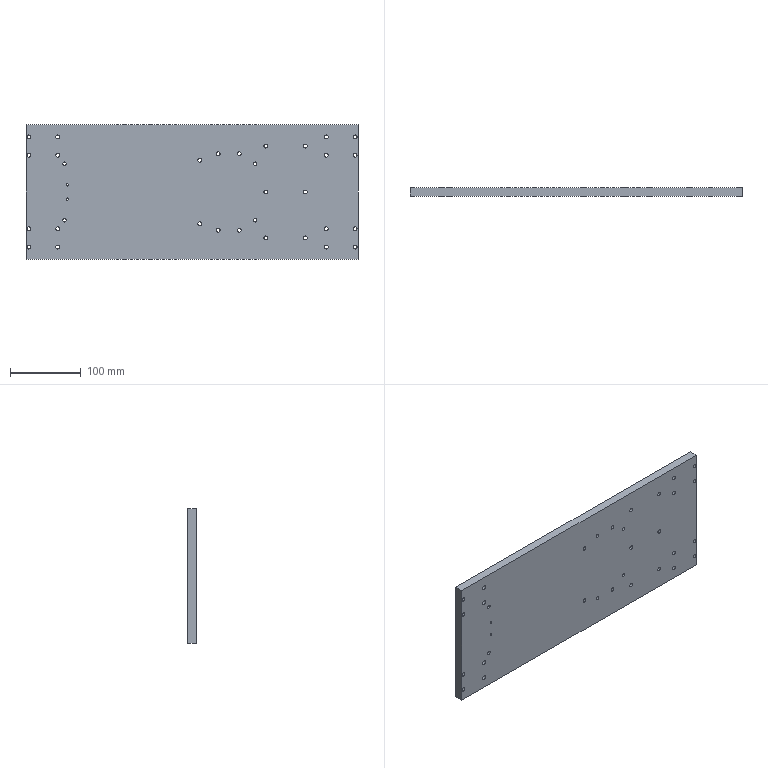Part | STEP file | 0245_209_Plate | 1 solid | 74 faces | box 470 x 12 x 190 mm | volume 1062469 mm3 | cylinder 68 | plane 6 | commonest cylinder face diameters 5.5 x56 5 x8 3.3 x4